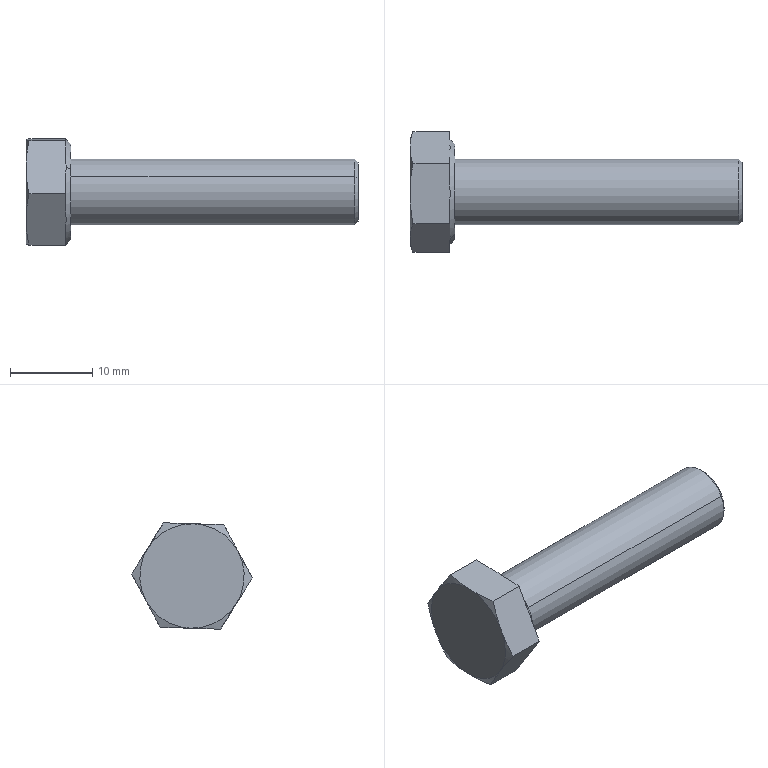Part | NX | features BREP 1 | 1 solid | 27 faces | box 40.45 x 14.692 x 12.962 mm | volume 2507 mm3 | plane 15 | cone 10 | cylinder 2 | commonest cylinder face diameters 8 x2
STEP:
#1=CARTESIAN_POINT('',(711.845,-32.743,42.746));
#2=VERTEX_POINT('',#1);
#3=CARTESIAN_POINT('',(711.845,-39.092,46.141));
#4=VERTEX_POINT('',#3);
#5=CARTESIAN_POINT('',(711.845,-35.917,44.443));
#6=DIRECTION('',(1.,0.,0.));
#7=DIRECTION('',(0.,0.8818,-0.4716));
#8=AXIS2_PLACEMENT_3D('',#5,#6,#7);
#9=CIRCLE('',#8,3.6);
#10=EDGE_CURVE('',#2,#4,#9,.T.);
#11=ORIENTED_EDGE('',*,*,#10,.F.);
#12=CARTESIAN_POINT('',(711.445,-32.39,42.557));
#13=VERTEX_POINT('',#12);
#14=CARTESIAN_POINT('',(711.845,-32.743,42.746));
#15=DIRECTION('',(-0.7071,0.6235,-0.3335));
#16=VECTOR('',#15,1000.);
#17=LINE('',#14,#16);
#18=EDGE_CURVE('',#13,#2,#17,.F.);
#19=ORIENTED_EDGE('',*,*,#18,.F.);
#20=CARTESIAN_POINT('',(711.445,-39.444,46.33));
#21=VERTEX_POINT('',#20);
#22=CARTESIAN_POINT('',(711.445,-35.917,44.443));
#23=DIRECTION('',(-1.,0.,0.));
#24=DIRECTION('',(0.,0.8818,-0.4716));
#25=AXIS2_PLACEMENT_3D('',#22,#23,#24);
#26=CIRCLE('',#25,4.);
#27=EDGE_CURVE('',#21,#13,#26,.T.);
#28=ORIENTED_EDGE('',*,*,#27,.F.);
#29=CARTESIAN_POINT('',(711.845,-39.092,46.141));
#30=DIRECTION('',(-0.7071,-0.6235,0.3335));
#31=VECTOR('',#30,1000.);
#32=LINE('',#29,#31);
#33=EDGE_CURVE('',#21,#4,#32,.F.);
#34=ORIENTED_EDGE('',*,*,#33,.T.);
#35=EDGE_LOOP('',(#11,#19,#28,#34));
#36=FACE_BOUND('',#35,.T.);
#37=CARTESIAN_POINT('',(711.845,-35.917,44.443));
#38=DIRECTION('',(-1.,0.,0.));
#39=DIRECTION('',(0.,0.8818,-0.4716));
#40=AXIS2_PLACEMENT_3D('',#37,#38,#39);
#41=CONICAL_SURFACE('',#40,3.6,0.7854);
#42=ADVANCED_FACE('',(#36),#41,.T.);
#43=ORIENTED_EDGE('',*,*,#27,.T.);
#44=CARTESIAN_POINT('',(676.845,-32.39,42.557));
#45=VERTEX_POINT('',#44);
#46=CARTESIAN_POINT('',(711.845,-32.39,42.557));
#47=DIRECTION('',(-1.,0.,0.));
#48=VECTOR('',#47,1000.);
#49=LINE('',#46,#48);
#50=EDGE_CURVE('',#45,#13,#49,.F.);
#51=ORIENTED_EDGE('',*,*,#50,.F.);
#52=CARTESIAN_POINT('',(676.845,-39.444,46.33));
#53=VERTEX_POINT('',#52);
#54=CARTESIAN_POINT('',(676.845,-35.917,44.443));
#55=DIRECTION('',(1.,0.,0.));
#56=DIRECTION('',(0.,0.8818,-0.4716));
#57=AXIS2_PLACEMENT_3D('',#54,#55,#56);
#58=CIRCLE('',#57,4.);
#59=EDGE_CURVE('',#45,#53,#58,.T.);
#60=ORIENTED_EDGE('',*,*,#59,.T.);
#61=CARTESIAN_POINT('',(711.845,-39.444,46.33));
#62=DIRECTION('',(-1.,0.,0.));
#63=VECTOR('',#62,1000.);
#64=LINE('',#61,#63);
#65=EDGE_CURVE('',#53,#21,#64,.F.);
#66=ORIENTED_EDGE('',*,*,#65,.T.);
#67=EDGE_LOOP('',(#43,#51,#60,#66));
#68=FACE_BOUND('',#67,.T.);
#69=CARTESIAN_POINT('',(711.845,-35.917,44.443));
#70=DIRECTION('',(-1.,0.,0.));
#71=DIRECTION('',(0.,0.8818,-0.4716));
#72=AXIS2_PLACEMENT_3D('',#69,#70,#71);
#73=CYLINDRICAL_SURFACE('',#72,4.);
#74=ADVANCED_FACE('',(#68),#73,.T.);
#75=CARTESIAN_POINT('',(676.845,-41.045,47.185));
#76=VERTEX_POINT('',#75);
#77=CARTESIAN_POINT('',(676.845,-30.789,41.701));
#78=VERTEX_POINT('',#77);
#79=CARTESIAN_POINT('',(676.845,-35.917,44.443));
#80=DIRECTION('',(-1.,0.,0.));
#81=DIRECTION('',(0.,-0.8818,0.4716));
#82=AXIS2_PLACEMENT_3D('',#79,#80,#81);
#83=CIRCLE('',#82,5.815);
#84=EDGE_CURVE('',#76,#78,#83,.T.);
#85=ORIENTED_EDGE('',*,*,#84,.T.);
#86=CARTESIAN_POINT('',(676.295,-30.304,41.442));
#87=VERTEX_POINT('',#86);
#88=CARTESIAN_POINT('',(676.245,-30.26,41.418));
#89=DIRECTION('',(-0.7071,0.6235,-0.3335));
#90=VECTOR('',#89,1000.);
#91=LINE('',#88,#90);
#92=EDGE_CURVE('',#87,#78,#91,.F.);
#93=ORIENTED_EDGE('',*,*,#92,.F.);
#94=CARTESIAN_POINT('',(676.245,-29.927,42.147));
#95=VERTEX_POINT('',#94);
#96=CARTESIAN_POINT('',(676.295,-30.304,41.442));
#97=CARTESIAN_POINT('',(676.295,-30.179,41.677));
#98=CARTESIAN_POINT('',(676.278,-30.053,41.912));
#99=CARTESIAN_POINT('',(676.245,-29.927,42.147));
#100=B_SPLINE_CURVE_WITH_KNOTS('',3,(#96,#97,#98,#99),.UNSPECIFIED.,.F.,.F.,(4,4),(0.,1.),.PIECEWISE_BEZIER_KNOTS.);
#101=EDGE_CURVE('',#87,#95,#100,.T.);
#102=ORIENTED_EDGE('',*,*,#101,.T.);
#103=CARTESIAN_POINT('',(676.245,-30.089,47.124));
#104=VERTEX_POINT('',#103);
#105=CARTESIAN_POINT('',(676.245,-35.917,44.443));
#106=DIRECTION('',(-1.,0.,0.));
#107=DIRECTION('',(0.,-0.8818,0.4716));
#108=AXIS2_PLACEMENT_3D('',#105,#106,#107);
#109=CIRCLE('',#108,6.415);
#110=EDGE_CURVE('',#104,#95,#109,.T.);
#111=ORIENTED_EDGE('',*,*,#110,.F.);
#112=CARTESIAN_POINT('',(676.245,-30.933,48.482));
#113=VERTEX_POINT('',#112);
#114=CARTESIAN_POINT('',(676.245,-30.089,47.124));
#115=CARTESIAN_POINT('',(676.311,-30.371,47.577));
#116=CARTESIAN_POINT('',(676.311,-30.652,48.03));
#117=CARTESIAN_POINT('',(676.245,-30.933,48.482));
#118=B_SPLINE_CURVE_WITH_KNOTS('',3,(#114,#115,#116,#117),.UNSPECIFIED.,.F.,.F.,(4,4),(0.,0.001599),.UNSPECIFIED.);
#119=EDGE_CURVE('',#104,#113,#118,.T.);
#120=ORIENTED_EDGE('',*,*,#119,.T.);
#121=CARTESIAN_POINT('',(676.245,-35.325,50.831));
#122=VERTEX_POINT('',#121);
#123=CARTESIAN_POINT('',(676.245,-35.917,44.443));
#124=DIRECTION('',(-1.,0.,0.));
#125=DIRECTION('',(0.,-0.8818,0.4716));
#126=AXIS2_PLACEMENT_3D('',#123,#124,#125);
#127=CIRCLE('',#126,6.415);
#128=EDGE_CURVE('',#122,#113,#127,.T.);
#129=ORIENTED_EDGE('',*,*,#128,.F.);
#130=CARTESIAN_POINT('',(676.245,-36.923,50.779));
#131=VERTEX_POINT('',#130);
#132=CARTESIAN_POINT('',(676.245,-35.325,50.831));
#133=CARTESIAN_POINT('',(676.311,-35.858,50.814));
#134=CARTESIAN_POINT('',(676.311,-36.391,50.796));
#135=CARTESIAN_POINT('',(676.245,-36.923,50.779));
#136=B_SPLINE_CURVE_WITH_KNOTS('',3,(#132,#133,#134,#135),.UNSPECIFIED.,.F.,.F.,(4,4),(0.,0.001599),.UNSPECIFIED.);
#137=EDGE_CURVE('',#122,#131,#136,.T.);
#138=ORIENTED_EDGE('',*,*,#137,.T.);
#139=CARTESIAN_POINT('',(676.245,-41.153,48.15));
#140=VERTEX_POINT('',#139);
#141=CARTESIAN_POINT('',(676.245,-35.917,44.443));
#142=DIRECTION('',(-1.,0.,0.));
#143=DIRECTION('',(0.,-0.8818,0.4716));
#144=AXIS2_PLACEMENT_3D('',#141,#142,#143);
#145=CIRCLE('',#144,6.415);
#146=EDGE_CURVE('',#140,#131,#145,.T.);
#147=ORIENTED_EDGE('',*,*,#146,.F.);
#148=CARTESIAN_POINT('',(676.295,-41.53,47.445));
#149=VERTEX_POINT('',#148);
#150=CARTESIAN_POINT('',(676.245,-41.153,48.15));
#151=CARTESIAN_POINT('',(676.278,-41.279,47.915));
#152=CARTESIAN_POINT('',(676.295,-41.404,47.68));
#153=CARTESIAN_POINT('',(676.295,-41.53,47.445));
#154=B_SPLINE_CURVE_WITH_KNOTS('',3,(#150,#151,#152,#153),.UNSPECIFIED.,.F.,.F.,(4,4),(0.,1.),.PIECEWISE_BEZIER_KNOTS.);
#155=EDGE_CURVE('',#140,#149,#154,.T.);
#156=ORIENTED_EDGE('',*,*,#155,.T.);
#157=CARTESIAN_POINT('',(676.245,-41.574,47.468));
#158=DIRECTION('',(-0.7071,-0.6235,0.3335));
#159=VECTOR('',#158,1000.);
#160=LINE('',#157,#159);
#161=EDGE_CURVE('',#149,#76,#160,.F.);
#162=ORIENTED_EDGE('',*,*,#161,.T.);
#163=EDGE_LOOP('',(#85,#93,#102,#111,#120,#129,#138,#147,#156,#162));
#164=FACE_BOUND('',#163,.T.);
#165=CARTESIAN_POINT('',(676.245,-35.917,44.443));
#166=DIRECTION('',(-1.,0.,0.));
#167=DIRECTION('',(0.,0.8818,-0.4716));
#168=AXIS2_PLACEMENT_3D('',#165,#166,#167);
#169=CONICAL_SURFACE('',#168,6.415,0.7854);
#170=ADVANCED_FACE('',(#164),#169,.T.);
#171=ORIENTED_EDGE('',*,*,#84,.F.);
#172=CARTESIAN_POINT('',(676.845,-35.917,44.443));
#173=DIRECTION('',(-1.,0.,0.));
#174=DIRECTION('',(0.,-0.8818,0.4716));
#175=AXIS2_PLACEMENT_3D('',#172,#173,#174);
#176=CIRCLE('',#175,5.815);
#177=EDGE_CURVE('',#78,#76,#176,.T.);
#178=ORIENTED_EDGE('',*,*,#177,.F.);
#179=EDGE_LOOP('',(#171,#178));
#180=FACE_BOUND('',#179,.T.);
#181=CARTESIAN_POINT('',(676.845,-35.917,44.443));
#182=DIRECTION('',(1.,0.,0.));
#183=DIRECTION('',(0.,0.8818,-0.4716));
#184=AXIS2_PLACEMENT_3D('',#181,#182,#183);
#185=CIRCLE('',#184,4.);
#186=EDGE_CURVE('',#53,#45,#185,.T.);
#187=ORIENTED_EDGE('',*,*,#186,.F.);
#188=ORIENTED_EDGE('',*,*,#59,.F.);
#189=EDGE_LOOP('',(#187,#188));
#190=FACE_BOUND('',#189,.T.);
#191=CARTESIAN_POINT('',(676.845,-32.037,38.201));
#192=DIRECTION('',(1.,0.,0.));
#193=DIRECTION('',(0.,-0.8818,0.4716));
#194=AXIS2_PLACEMENT_3D('',#191,#192,#193);
#195=PLANE('',#194);
#196=ADVANCED_FACE('',(#180,#190),#195,.T.);
#197=CARTESIAN_POINT('',(671.753,-32.037,38.201));
#198=VERTEX_POINT('',#197);
#199=CARTESIAN_POINT('',(671.395,-35.71,38.082));
#200=VERTEX_POINT('',#199);
#201=CARTESIAN_POINT('',(671.753,-32.037,38.201));
#202=CARTESIAN_POINT('',(671.532,-33.252,38.162));
#203=CARTESIAN_POINT('',(671.395,-34.474,38.122));
#204=CARTESIAN_POINT('',(671.395,-35.71,38.082));
#205=B_SPLINE_CURVE_WITH_KNOTS('',3,(#201,#202,#203,#204),.UNSPECIFIED.,.F.,.F.,(4,4),(0.,0.003692),.UNSPECIFIED.);
#206=EDGE_CURVE('',#198,#200,#205,.T.);
#207=ORIENTED_EDGE('',*,*,#206,.F.);
#208=CARTESIAN_POINT('',(676.245,-32.037,38.201));
#209=VERTEX_POINT('',#208);
#210=CARTESIAN_POINT('',(676.845,-32.037,38.201));
#211=DIRECTION('',(-1.,0.,0.));
#212=VECTOR('',#211,1000.);
#213=LINE('',#210,#212);
#214=EDGE_CURVE('',#209,#198,#213,.T.);
#215=ORIENTED_EDGE('',*,*,#214,.F.);
#216=CARTESIAN_POINT('',(676.245,-34.911,38.108));
#217=VERTEX_POINT('',#216);
#218=CARTESIAN_POINT('',(676.245,-39.383,37.962));
#219=DIRECTION('',(0.,0.9995,0.03252));
#220=VECTOR('',#219,1000.);
#221=LINE('',#218,#220);
#222=EDGE_CURVE('',#217,#209,#221,.T.);
#223=ORIENTED_EDGE('',*,*,#222,.F.);
#224=CARTESIAN_POINT('',(676.245,-36.509,38.056));
#225=VERTEX_POINT('',#224);
#226=CARTESIAN_POINT('',(676.245,-36.509,38.056));
#227=CARTESIAN_POINT('',(676.311,-35.976,38.073));
#228=CARTESIAN_POINT('',(676.311,-35.444,38.09));
#229=CARTESIAN_POINT('',(676.245,-34.911,38.108));
#230=B_SPLINE_CURVE_WITH_KNOTS('',3,(#226,#227,#228,#229),.UNSPECIFIED.,.F.,.F.,(4,4),(0.,0.001599),.UNSPECIFIED.);
#231=EDGE_CURVE('',#225,#217,#230,.T.);
#232=ORIENTED_EDGE('',*,*,#231,.F.);
#233=CARTESIAN_POINT('',(676.245,-39.383,37.962));
#234=VERTEX_POINT('',#233);
#235=CARTESIAN_POINT('',(676.245,-39.383,37.962));
#236=DIRECTION('',(0.,0.9995,0.03252));
#237=VECTOR('',#236,1000.);
#238=LINE('',#235,#237);
#239=EDGE_CURVE('',#234,#225,#238,.T.);
#240=ORIENTED_EDGE('',*,*,#239,.F.);
#241=CARTESIAN_POINT('',(671.753,-39.383,37.962));
#242=VERTEX_POINT('',#241);
#243=CARTESIAN_POINT('',(676.845,-39.383,37.962));
#244=DIRECTION('',(-1.,0.,0.));
#245=VECTOR('',#244,1000.);
#246=LINE('',#243,#245);
#247=EDGE_CURVE('',#234,#242,#246,.T.);
#248=ORIENTED_EDGE('',*,*,#247,.T.);
#249=CARTESIAN_POINT('',(671.395,-35.71,38.082));
#250=CARTESIAN_POINT('',(671.395,-36.946,38.041));
#251=CARTESIAN_POINT('',(671.532,-38.169,38.002));
#252=CARTESIAN_POINT('',(671.753,-39.383,37.962));
#253=B_SPLINE_CURVE_WITH_KNOTS('',3,(#249,#250,#251,#252),.UNSPECIFIED.,.F.,.F.,(4,4),(0.,0.003692),.UNSPECIFIED.);
#254=EDGE_CURVE('',#200,#242,#253,.T.);
#255=ORIENTED_EDGE('',*,*,#254,.F.);
#256=EDGE_LOOP('',(#207,#215,#223,#232,#240,#248,#255));
#257=FACE_BOUND('',#256,.T.);
#258=CARTESIAN_POINT('',(676.845,-39.383,37.962));
#259=DIRECTION('',(0.,-0.03252,0.9995));
#260=DIRECTION('',(0.,0.9995,0.03252));
#261=AXIS2_PLACEMENT_3D('',#258,#259,#260);
#262=PLANE('',#261);
#263=ADVANCED_FACE('',(#257),#262,.F.);
#264=CARTESIAN_POINT('',(671.753,-28.571,44.682));
#265=VERTEX_POINT('',#264);
#266=CARTESIAN_POINT('',(671.395,-30.304,41.442));
#267=VERTEX_POINT('',#266);
#268=CARTESIAN_POINT('',(671.753,-28.571,44.682));
#269=CARTESIAN_POINT('',(671.532,-29.144,43.611));
#270=CARTESIAN_POINT('',(671.395,-29.721,42.532));
#271=CARTESIAN_POINT('',(671.395,-30.304,41.442));
#272=B_SPLINE_CURVE_WITH_KNOTS('',3,(#268,#269,#270,#271),.UNSPECIFIED.,.F.,.F.,(4,4),(0.,0.003692),.UNSPECIFIED.);
#273=EDGE_CURVE('',#265,#267,#272,.T.);
#274=ORIENTED_EDGE('',*,*,#273,.F.);
#275=CARTESIAN_POINT('',(676.245,-28.571,44.682));
#276=VERTEX_POINT('',#275);
#277=CARTESIAN_POINT('',(676.845,-28.571,44.682));
#278=DIRECTION('',(-1.,0.,0.));
#279=VECTOR('',#278,1000.);
#280=LINE('',#277,#279);
#281=EDGE_CURVE('',#276,#265,#280,.T.);
#282=ORIENTED_EDGE('',*,*,#281,.F.);
#283=CARTESIAN_POINT('',(676.245,-32.037,38.201));
#284=DIRECTION('',(0.,0.4716,0.8818));
#285=VECTOR('',#284,1000.);
#286=LINE('',#283,#285);
#287=EDGE_CURVE('',#95,#276,#286,.T.);
#288=ORIENTED_EDGE('',*,*,#287,.F.);
#289=ORIENTED_EDGE('',*,*,#101,.F.);
#290=CARTESIAN_POINT('',(676.245,-30.681,40.737));
#291=VERTEX_POINT('',#290);
#292=CARTESIAN_POINT('',(676.245,-30.681,40.737));
#293=CARTESIAN_POINT('',(676.278,-30.556,40.972));
#294=CARTESIAN_POINT('',(676.295,-30.43,41.207));
#295=CARTESIAN_POINT('',(676.295,-30.304,41.442));
#296=B_SPLINE_CURVE_WITH_KNOTS('',3,(#292,#293,#294,#295),.UNSPECIFIED.,.F.,.F.,(4,4),(0.,1.),.PIECEWISE_BEZIER_KNOTS.);
#297=EDGE_CURVE('',#291,#87,#296,.T.);
#298=ORIENTED_EDGE('',*,*,#297,.F.);
#299=CARTESIAN_POINT('',(676.245,-32.037,38.201));
#300=DIRECTION('',(0.,0.4716,0.8818));
#301=VECTOR('',#300,1000.);
#302=LINE('',#299,#301);
#303=EDGE_CURVE('',#209,#291,#302,.T.);
#304=ORIENTED_EDGE('',*,*,#303,.F.);
#305=ORIENTED_EDGE('',*,*,#214,.T.);
#306=CARTESIAN_POINT('',(671.395,-30.304,41.442));
#307=CARTESIAN_POINT('',(671.395,-30.887,40.351));
#308=CARTESIAN_POINT('',(671.532,-31.464,39.273));
#309=CARTESIAN_POINT('',(671.753,-32.037,38.201));
#310=B_SPLINE_CURVE_WITH_KNOTS('',3,(#306,#307,#308,#309),.UNSPECIFIED.,.F.,.F.,(4,4),(0.,0.003692),.UNSPECIFIED.);
#311=EDGE_CURVE('',#267,#198,#310,.T.);
#312=ORIENTED_EDGE('',*,*,#311,.F.);
#313=EDGE_LOOP('',(#274,#282,#288,#289,#298,#304,#305,#312));
#314=FACE_BOUND('',#313,.T.);
#315=CARTESIAN_POINT('',(676.845,-32.037,38.201));
#316=DIRECTION('',(0.,-0.8818,0.4716));
#317=DIRECTION('',(-1.,0.,0.));
#318=AXIS2_PLACEMENT_3D('',#315,#316,#317);
#319=PLANE('',#318);
#320=ADVANCED_FACE('',(#314),#319,.F.);
#321=CARTESIAN_POINT('',(671.753,-32.451,50.924));
#322=VERTEX_POINT('',#321);
#323=CARTESIAN_POINT('',(671.395,-30.511,47.803));
#324=VERTEX_POINT('',#323);
#325=CARTESIAN_POINT('',(671.753,-32.451,50.924));
#326=CARTESIAN_POINT('',(671.532,-31.81,49.893));
#327=CARTESIAN_POINT('',(671.395,-31.164,48.854));
#328=CARTESIAN_POINT('',(671.395,-30.511,47.803));
#329=B_SPLINE_CURVE_WITH_KNOTS('',3,(#325,#326,#327,#328),.UNSPECIFIED.,.F.,.F.,(4,4),(0.,0.003692),.UNSPECIFIED.);
#330=EDGE_CURVE('',#322,#324,#329,.T.);
#331=ORIENTED_EDGE('',*,*,#330,.F.);
#332=CARTESIAN_POINT('',(676.245,-32.451,50.924));
#333=VERTEX_POINT('',#332);
#334=CARTESIAN_POINT('',(676.845,-32.451,50.924));
#335=DIRECTION('',(-1.,0.,0.));
#336=VECTOR('',#335,1000.);
#337=LINE('',#334,#336);
#338=EDGE_CURVE('',#333,#322,#337,.T.);
#339=ORIENTED_EDGE('',*,*,#338,.F.);
#340=CARTESIAN_POINT('',(676.245,-28.571,44.682));
#341=DIRECTION('',(0.,-0.5279,0.8493));
#342=VECTOR('',#341,1000.);
#343=LINE('',#340,#342);
#344=EDGE_CURVE('',#113,#333,#343,.T.);
#345=ORIENTED_EDGE('',*,*,#344,.F.);
#346=ORIENTED_EDGE('',*,*,#119,.F.);
#347=CARTESIAN_POINT('',(676.245,-28.571,44.682));
#348=DIRECTION('',(0.,-0.5279,0.8493));
#349=VECTOR('',#348,1000.);
#350=LINE('',#347,#349);
#351=EDGE_CURVE('',#276,#104,#350,.T.);
#352=ORIENTED_EDGE('',*,*,#351,.F.);
#353=ORIENTED_EDGE('',*,*,#281,.T.);
#354=CARTESIAN_POINT('',(671.395,-30.511,47.803));
#355=CARTESIAN_POINT('',(671.395,-29.859,46.753));
#356=CARTESIAN_POINT('',(671.532,-29.213,45.714));
#357=CARTESIAN_POINT('',(671.753,-28.571,44.682));
#358=B_SPLINE_CURVE_WITH_KNOTS('',3,(#354,#355,#356,#357),.UNSPECIFIED.,.F.,.F.,(4,4),(0.,0.003692),.UNSPECIFIED.);
#359=EDGE_CURVE('',#324,#265,#358,.T.);
#360=ORIENTED_EDGE('',*,*,#359,.F.);
#361=EDGE_LOOP('',(#331,#339,#345,#346,#352,#353,#360));
#362=FACE_BOUND('',#361,.T.);
#363=CARTESIAN_POINT('',(676.845,-28.571,44.682));
#364=DIRECTION('',(0.,-0.8493,-0.5279));
#365=DIRECTION('',(0.,-0.5279,0.8493));
#366=AXIS2_PLACEMENT_3D('',#363,#364,#365);
#367=PLANE('',#366);
#368=ADVANCED_FACE('',(#362),#367,.F.);
#369=CARTESIAN_POINT('',(671.753,-39.797,50.685));
#370=VERTEX_POINT('',#369);
#371=CARTESIAN_POINT('',(671.395,-36.124,50.805));
#372=VERTEX_POINT('',#371);
#373=CARTESIAN_POINT('',(671.753,-39.797,50.685));
#374=CARTESIAN_POINT('',(671.532,-38.583,50.725));
#375=CARTESIAN_POINT('',(671.395,-37.36,50.765));
#376=CARTESIAN_POINT('',(671.395,-36.124,50.805));
#377=B_SPLINE_CURVE_WITH_KNOTS('',3,(#373,#374,#375,#376),.UNSPECIFIED.,.F.,.F.,(4,4),(0.,0.003692),.UNSPECIFIED.);
#378=EDGE_CURVE('',#370,#372,#377,.T.);
#379=ORIENTED_EDGE('',*,*,#378,.F.);
#380=CARTESIAN_POINT('',(676.245,-39.797,50.685));
#381=VERTEX_POINT('',#380);
#382=CARTESIAN_POINT('',(676.845,-39.797,50.685));
#383=DIRECTION('',(-1.,0.,0.));
#384=VECTOR('',#383,1000.);
#385=LINE('',#382,#384);
#386=EDGE_CURVE('',#381,#370,#385,.T.);
#387=ORIENTED_EDGE('',*,*,#386,.F.);
#388=CARTESIAN_POINT('',(676.245,-32.451,50.924));
#389=DIRECTION('',(0.,-0.9995,-0.03252));
#390=VECTOR('',#389,1000.);
#391=LINE('',#388,#390);
#392=EDGE_CURVE('',#131,#381,#391,.T.);
#393=ORIENTED_EDGE('',*,*,#392,.F.);
#394=ORIENTED_EDGE('',*,*,#137,.F.);
#395=CARTESIAN_POINT('',(676.245,-32.451,50.924));
#396=DIRECTION('',(0.,-0.9995,-0.03252));
#397=VECTOR('',#396,1000.);
#398=LINE('',#395,#397);
#399=EDGE_CURVE('',#333,#122,#398,.T.);
#400=ORIENTED_EDGE('',*,*,#399,.F.);
#401=ORIENTED_EDGE('',*,*,#338,.T.);
#402=CARTESIAN_POINT('',(671.395,-36.124,50.805));
#403=CARTESIAN_POINT('',(671.395,-34.888,50.845));
#404=CARTESIAN_POINT('',(671.532,-33.666,50.885));
#405=CARTESIAN_POINT('',(671.753,-32.451,50.924));
#406=B_SPLINE_CURVE_WITH_KNOTS('',3,(#402,#403,#404,#405),.UNSPECIFIED.,.F.,.F.,(4,4),(0.,0.003692),.UNSPECIFIED.);
#407=EDGE_CURVE('',#372,#322,#406,.T.);
#408=ORIENTED_EDGE('',*,*,#407,.F.);
#409=EDGE_LOOP('',(#379,#387,#393,#394,#400,#401,#408));
#410=FACE_BOUND('',#409,.T.);
#411=CARTESIAN_POINT('',(676.845,-32.451,50.924));
#412=DIRECTION('',(0.,0.03252,-0.9995));
#413=DIRECTION('',(0.,-0.9995,-0.03252));
#414=AXIS2_PLACEMENT_3D('',#411,#412,#413);
#415=PLANE('',#414);
#416=ADVANCED_FACE('',(#410),#415,.F.);
#417=CARTESIAN_POINT('',(671.753,-43.263,44.204));
#418=VERTEX_POINT('',#417);
#419=CARTESIAN_POINT('',(671.395,-41.53,47.445));
#420=VERTEX_POINT('',#419);
#421=CARTESIAN_POINT('',(671.753,-43.263,44.204));
#422=CARTESIAN_POINT('',(671.532,-42.69,45.276));
#423=CARTESIAN_POINT('',(671.395,-42.113,46.354));
#424=CARTESIAN_POINT('',(671.395,-41.53,47.445));
#425=B_SPLINE_CURVE_WITH_KNOTS('',3,(#421,#422,#423,#424),.UNSPECIFIED.,.F.,.F.,(4,4),(0.,0.003692),.UNSPECIFIED.);
#426=EDGE_CURVE('',#418,#420,#425,.T.);
#427=ORIENTED_EDGE('',*,*,#426,.F.);
#428=CARTESIAN_POINT('',(676.245,-43.263,44.204));
#429=VERTEX_POINT('',#428);
#430=CARTESIAN_POINT('',(676.845,-43.263,44.204));
#431=DIRECTION('',(-1.,0.,0.));
#432=VECTOR('',#431,1000.);
#433=LINE('',#430,#432);
#434=EDGE_CURVE('',#429,#418,#433,.T.);
#435=ORIENTED_EDGE('',*,*,#434,.F.);
#436=CARTESIAN_POINT('',(676.245,-41.907,46.74));
#437=VERTEX_POINT('',#436);
#438=CARTESIAN_POINT('',(676.245,-39.797,50.685));
#439=DIRECTION('',(0.,-0.4716,-0.8818));
#440=VECTOR('',#439,1000.);
#441=LINE('',#438,#440);
#442=EDGE_CURVE('',#437,#429,#441,.T.);
#443=ORIENTED_EDGE('',*,*,#442,.F.);
#444=CARTESIAN_POINT('',(676.295,-41.53,47.445));
#445=CARTESIAN_POINT('',(676.295,-41.656,47.21));
#446=CARTESIAN_POINT('',(676.278,-41.781,46.975));
#447=CARTESIAN_POINT('',(676.245,-41.907,46.74));
#448=B_SPLINE_CURVE_WITH_KNOTS('',3,(#444,#445,#446,#447),.UNSPECIFIED.,.F.,.F.,(4,4),(0.,1.),.PIECEWISE_BEZIER_KNOTS.);
#449=EDGE_CURVE('',#149,#437,#448,.T.);
#450=ORIENTED_EDGE('',*,*,#449,.F.);
#451=ORIENTED_EDGE('',*,*,#155,.F.);
#452=CARTESIAN_POINT('',(676.245,-39.797,50.685));
#453=DIRECTION('',(0.,-0.4716,-0.8818));
#454=VECTOR('',#453,1000.);
#455=LINE('',#452,#454);
#456=EDGE_CURVE('',#381,#140,#455,.T.);
#457=ORIENTED_EDGE('',*,*,#456,.F.);
#458=ORIENTED_EDGE('',*,*,#386,.T.);
#459=CARTESIAN_POINT('',(671.395,-41.53,47.445));
#460=CARTESIAN_POINT('',(671.395,-40.947,48.535));
#461=CARTESIAN_POINT('',(671.532,-40.37,49.614));
#462=CARTESIAN_POINT('',(671.753,-39.797,50.685));
#463=B_SPLINE_CURVE_WITH_KNOTS('',3,(#459,#460,#461,#462),.UNSPECIFIED.,.F.,.F.,(4,4),(0.,0.003692),.UNSPECIFIED.);
#464=EDGE_CURVE('',#420,#370,#463,.T.);
#465=ORIENTED_EDGE('',*,*,#464,.F.);
#466=EDGE_LOOP('',(#427,#435,#443,#450,#451,#457,#458,#465));
#467=FACE_BOUND('',#466,.T.);
#468=CARTESIAN_POINT('',(676.845,-39.797,50.685));
#469=DIRECTION('',(0.,0.8818,-0.4716));
#470=DIRECTION('',(1.,0.,0.));
#471=AXIS2_PLACEMENT_3D('',#468,#469,#470);
#472=PLANE('',#471);
#473=ADVANCED_FACE('',(#467),#472,.F.);
#474=CARTESIAN_POINT('',(671.395,-41.323,41.083));
#475=VERTEX_POINT('',#474);
#476=CARTESIAN_POINT('',(671.753,-39.383,37.962));
#477=CARTESIAN_POINT('',(671.532,-40.024,38.994));
#478=CARTESIAN_POINT('',(671.395,-40.67,40.033));
#479=CARTESIAN_POINT('',(671.395,-41.323,41.083));
#480=B_SPLINE_CURVE_WITH_KNOTS('',3,(#476,#477,#478,#479),.UNSPECIFIED.,.F.,.F.,(4,4),(0.,0.003692),.UNSPECIFIED.);
#481=EDGE_CURVE('',#242,#475,#480,.T.);
#482=ORIENTED_EDGE('',*,*,#481,.F.);
#483=ORIENTED_EDGE('',*,*,#247,.F.);
#484=CARTESIAN_POINT('',(676.245,-40.901,40.404));
#485=VERTEX_POINT('',#484);
#486=CARTESIAN_POINT('',(676.245,-43.263,44.204));
#487=DIRECTION('',(0.,0.5279,-0.8493));
#488=VECTOR('',#487,1000.);
#489=LINE('',#486,#488);
#490=EDGE_CURVE('',#485,#234,#489,.T.);
#491=ORIENTED_EDGE('',*,*,#490,.F.);
#492=CARTESIAN_POINT('',(676.245,-41.745,41.762));
#493=VERTEX_POINT('',#492);
#494=CARTESIAN_POINT('',(676.245,-41.745,41.762));
#495=CARTESIAN_POINT('',(676.311,-41.464,41.31));
#496=CARTESIAN_POINT('',(676.311,-41.182,40.857));
#497=CARTESIAN_POINT('',(676.245,-40.901,40.404));
#498=B_SPLINE_CURVE_WITH_KNOTS('',3,(#494,#495,#496,#497),.UNSPECIFIED.,.F.,.F.,(4,4),(0.,0.001599),.UNSPECIFIED.);
#499=EDGE_CURVE('',#493,#485,#498,.T.);
#500=ORIENTED_EDGE('',*,*,#499,.F.);
#501=CARTESIAN_POINT('',(676.245,-43.263,44.204));
#502=DIRECTION('',(0.,0.5279,-0.8493));
#503=VECTOR('',#502,1000.);
#504=LINE('',#501,#503);
#505=EDGE_CURVE('',#429,#493,#504,.T.);
#506=ORIENTED_EDGE('',*,*,#505,.F.);
#507=ORIENTED_EDGE('',*,*,#434,.T.);
#508=CARTESIAN_POINT('',(671.395,-41.323,41.083));
#509=CARTESIAN_POINT('',(671.395,-41.976,42.133));
#510=CARTESIAN_POINT('',(671.532,-42.622,43.172));
#511=CARTESIAN_POINT('',(671.753,-43.263,44.204));
#512=B_SPLINE_CURVE_WITH_KNOTS('',3,(#508,#509,#510,#511),.UNSPECIFIED.,.F.,.F.,(4,4),(0.,0.003692),.UNSPECIFIED.);
#513=EDGE_CURVE('',#475,#418,#512,.T.);
#514=ORIENTED_EDGE('',*,*,#513,.F.);
#515=EDGE_LOOP('',(#482,#483,#491,#500,#506,#507,#514));
#516=FACE_BOUND('',#515,.T.);
#517=CARTESIAN_POINT('',(676.845,-43.263,44.204));
#518=DIRECTION('',(0.,0.8493,0.5279));
#519=DIRECTION('',(0.,0.5279,-0.8493));
#520=AXIS2_PLACEMENT_3D('',#517,#518,#519);
#521=PLANE('',#520);
#522=ADVANCED_FACE('',(#516),#521,.F.);
#523=ORIENTED_EDGE('',*,*,#222,.T.);
#524=ORIENTED_EDGE('',*,*,#303,.T.);
#525=CARTESIAN_POINT('',(676.245,-35.917,44.443));
#526=DIRECTION('',(-1.,0.,0.));
#527=DIRECTION('',(0.,-0.8818,0.4716));
#528=AXIS2_PLACEMENT_3D('',#525,#526,#527);
#529=CIRCLE('',#528,6.415);
#530=EDGE_CURVE('',#291,#217,#529,.T.);
#531=ORIENTED_EDGE('',*,*,#530,.T.);
#532=EDGE_LOOP('',(#523,#524,#531));
#533=FACE_BOUND('',#532,.T.);
#534=CARTESIAN_POINT('',(676.245,-32.892,50.1));
#535=DIRECTION('',(1.,0.,0.));
#536=DIRECTION('',(0.,-0.8818,0.4716));
#537=AXIS2_PLACEMENT_3D('',#534,#535,#536);
#538=PLANE('',#537);
#539=ADVANCED_FACE('',(#533),#538,.T.);
#540=ORIENTED_EDGE('',*,*,#287,.T.);
#541=ORIENTED_EDGE('',*,*,#351,.T.);
#542=ORIENTED_EDGE('',*,*,#110,.T.);
#543=EDGE_LOOP('',(#540,#541,#542));
#544=FACE_BOUND('',#543,.T.);
#545=CARTESIAN_POINT('',(676.245,-32.892,50.1));
#546=DIRECTION('',(1.,0.,0.));
#547=DIRECTION('',(0.,-0.8818,0.4716));
#548=AXIS2_PLACEMENT_3D('',#545,#546,#547);
#549=PLANE('',#548);
#550=ADVANCED_FACE('',(#544),#549,.T.);
#551=ORIENTED_EDGE('',*,*,#344,.T.);
#552=ORIENTED_EDGE('',*,*,#399,.T.);
#553=ORIENTED_EDGE('',*,*,#128,.T.);
#554=EDGE_LOOP('',(#551,#552,#553));
#555=FACE_BOUND('',#554,.T.);
#556=CARTESIAN_POINT('',(676.245,-32.892,50.1));
#557=DIRECTION('',(1.,0.,0.));
#558=DIRECTION('',(0.,-0.8818,0.4716));
#559=AXIS2_PLACEMENT_3D('',#556,#557,#558);
#560=PLANE('',#559);
#561=ADVANCED_FACE('',(#555),#560,.T.);
#562=ORIENTED_EDGE('',*,*,#392,.T.);
#563=ORIENTED_EDGE('',*,*,#456,.T.);
#564=ORIENTED_EDGE('',*,*,#146,.T.);
#565=EDGE_LOOP('',(#562,#563,#564));
#566=FACE_BOUND('',#565,.T.);
#567=CARTESIAN_POINT('',(676.245,-32.892,50.1));
#568=DIRECTION('',(1.,0.,0.));
#569=DIRECTION('',(0.,-0.8818,0.4716));
#570=AXIS2_PLACEMENT_3D('',#567,#568,#569);
#571=PLANE('',#570);
#572=ADVANCED_FACE('',(#566),#571,.T.);
#573=ORIENTED_EDGE('',*,*,#442,.T.);
#574=ORIENTED_EDGE('',*,*,#505,.T.);
#575=CARTESIAN_POINT('',(676.245,-35.917,44.443));
#576=DIRECTION('',(-1.,0.,0.));
#577=DIRECTION('',(0.,-0.8818,0.4716));
#578=AXIS2_PLACEMENT_3D('',#575,#576,#577);
#579=CIRCLE('',#578,6.415);
#580=EDGE_CURVE('',#493,#437,#579,.T.);
#581=ORIENTED_EDGE('',*,*,#580,.T.);
#582=EDGE_LOOP('',(#573,#574,#581));
#583=FACE_BOUND('',#582,.T.);
#584=CARTESIAN_POINT('',(676.245,-32.892,50.1));
#585=DIRECTION('',(1.,0.,0.));
#586=DIRECTION('',(0.,-0.8818,0.4716));
#587=AXIS2_PLACEMENT_3D('',#584,#585,#586);
#588=PLANE('',#587);
#589=ADVANCED_FACE('',(#583),#588,.T.);
#590=ORIENTED_EDGE('',*,*,#239,.T.);
#591=CARTESIAN_POINT('',(676.245,-35.917,44.443));
#592=DIRECTION('',(-1.,0.,0.));
#593=DIRECTION('',(0.,-0.8818,0.4716));
#594=AXIS2_PLACEMENT_3D('',#591,#592,#593);
#595=CIRCLE('',#594,6.415);
#596=EDGE_CURVE('',#225,#485,#595,.T.);
#597=ORIENTED_EDGE('',*,*,#596,.T.);
#598=ORIENTED_EDGE('',*,*,#490,.T.);
#599=EDGE_LOOP('',(#590,#597,#598));
#600=FACE_BOUND('',#599,.T.);
#601=CARTESIAN_POINT('',(676.245,-32.892,50.1));
#602=DIRECTION('',(1.,0.,0.));
#603=DIRECTION('',(0.,-0.8818,0.4716));
#604=AXIS2_PLACEMENT_3D('',#601,#602,#603);
#605=PLANE('',#604);
#606=ADVANCED_FACE('',(#600),#605,.T.);
#607=ORIENTED_EDGE('',*,*,#92,.T.);
#608=ORIENTED_EDGE('',*,*,#177,.T.);
#609=ORIENTED_EDGE('',*,*,#161,.F.);
#610=ORIENTED_EDGE('',*,*,#449,.T.);
#611=ORIENTED_EDGE('',*,*,#580,.F.);
#612=ORIENTED_EDGE('',*,*,#499,.T.);
#613=ORIENTED_EDGE('',*,*,#596,.F.);
#614=ORIENTED_EDGE('',*,*,#231,.T.);
#615=ORIENTED_EDGE('',*,*,#530,.F.);
#616=ORIENTED_EDGE('',*,*,#297,.T.);
#617=EDGE_LOOP('',(#607,#608,#609,#610,#611,#612,#613,#614,#615,#616));
#618=FACE_BOUND('',#617,.T.);
#619=CARTESIAN_POINT('',(676.245,-35.917,44.443));
#620=DIRECTION('',(-1.,0.,0.));
#621=DIRECTION('',(0.,0.8818,-0.4716));
#622=AXIS2_PLACEMENT_3D('',#619,#620,#621);
#623=CONICAL_SURFACE('',#622,6.415,0.7854);
#624=ADVANCED_FACE('',(#618),#623,.T.);
#625=ORIENTED_EDGE('',*,*,#311,.T.);
#626=ORIENTED_EDGE('',*,*,#206,.T.);
#627=CARTESIAN_POINT('',(671.395,-35.917,44.443));
#628=DIRECTION('',(1.,0.,0.));
#629=DIRECTION('',(0.,0.8818,-0.4716));
#630=AXIS2_PLACEMENT_3D('',#627,#628,#629);
#631=CIRCLE('',#630,6.365);
#632=EDGE_CURVE('',#200,#267,#631,.T.);
#633=ORIENTED_EDGE('',*,*,#632,.T.);
#634=EDGE_LOOP('',(#625,#626,#633));
#635=FACE_BOUND('',#634,.T.);
#636=CARTESIAN_POINT('',(671.395,-35.917,44.443));
#637=DIRECTION('',(1.,0.,0.));
#638=DIRECTION('',(0.,-0.8818,0.4716));
#639=AXIS2_PLACEMENT_3D('',#636,#637,#638);
#640=CONICAL_SURFACE('',#639,6.365,1.222);
#641=ADVANCED_FACE('',(#635),#640,.T.);
#642=ORIENTED_EDGE('',*,*,#254,.T.);
#643=ORIENTED_EDGE('',*,*,#481,.T.);
#644=CARTESIAN_POINT('',(671.395,-35.917,44.443));
#645=DIRECTION('',(1.,0.,0.));
#646=DIRECTION('',(0.,0.8818,-0.4716));
#647=AXIS2_PLACEMENT_3D('',#644,#645,#646);
#648=CIRCLE('',#647,6.365);
#649=EDGE_CURVE('',#475,#200,#648,.T.);
#650=ORIENTED_EDGE('',*,*,#649,.T.);
#651=EDGE_LOOP('',(#642,#643,#650));
#652=FACE_BOUND('',#651,.T.);
#653=CARTESIAN_POINT('',(671.395,-35.917,44.443));
#654=DIRECTION('',(1.,0.,0.));
#655=DIRECTION('',(0.,-0.8818,0.4716));
#656=AXIS2_PLACEMENT_3D('',#653,#654,#655);
#657=CONICAL_SURFACE('',#656,6.365,1.222);
#658=ADVANCED_FACE('',(#652),#657,.T.);
#659=ORIENTED_EDGE('',*,*,#426,.T.);
#660=CARTESIAN_POINT('',(671.395,-35.917,44.443));
#661=DIRECTION('',(1.,0.,0.));
#662=DIRECTION('',(0.,0.8818,-0.4716));
#663=AXIS2_PLACEMENT_3D('',#660,#661,#662);
#664=CIRCLE('',#663,6.365);
#665=EDGE_CURVE('',#420,#475,#664,.T.);
#666=ORIENTED_EDGE('',*,*,#665,.T.);
#667=ORIENTED_EDGE('',*,*,#513,.T.);
#668=EDGE_LOOP('',(#659,#666,#667));
#669=FACE_BOUND('',#668,.T.);
#670=CARTESIAN_POINT('',(671.395,-35.917,44.443));
#671=DIRECTION('',(1.,0.,0.));
#672=DIRECTION('',(0.,-0.8818,0.4716));
#673=AXIS2_PLACEMENT_3D('',#670,#671,#672);
#674=CONICAL_SURFACE('',#673,6.365,1.222);
#675=ADVANCED_FACE('',(#669),#674,.T.);
#676=ORIENTED_EDGE('',*,*,#378,.T.);
#677=CARTESIAN_POINT('',(671.395,-35.917,44.443));
#678=DIRECTION('',(-1.,0.,0.));
#679=DIRECTION('',(0.,-0.8818,0.4716));
#680=AXIS2_PLACEMENT_3D('',#677,#678,#679);
#681=CIRCLE('',#680,6.365);
#682=EDGE_CURVE('',#420,#372,#681,.T.);
#683=ORIENTED_EDGE('',*,*,#682,.F.);
#684=ORIENTED_EDGE('',*,*,#464,.T.);
#685=EDGE_LOOP('',(#676,#683,#684));
#686=FACE_BOUND('',#685,.T.);
#687=CARTESIAN_POINT('',(671.395,-35.917,44.443));
#688=DIRECTION('',(1.,0.,0.));
#689=DIRECTION('',(0.,-0.8818,0.4716));
#690=AXIS2_PLACEMENT_3D('',#687,#688,#689);
#691=CONICAL_SURFACE('',#690,6.365,1.222);
#692=ADVANCED_FACE('',(#686),#691,.T.);
#693=ORIENTED_EDGE('',*,*,#330,.T.);
#694=CARTESIAN_POINT('',(671.395,-35.917,44.443));
#695=DIRECTION('',(1.,0.,0.));
#696=DIRECTION('',(0.,0.8818,-0.4716));
#697=AXIS2_PLACEMENT_3D('',#694,#695,#696);
#698=CIRCLE('',#697,6.365);
#699=EDGE_CURVE('',#324,#372,#698,.T.);
#700=ORIENTED_EDGE('',*,*,#699,.T.);
#701=ORIENTED_EDGE('',*,*,#407,.T.);
#702=EDGE_LOOP('',(#693,#700,#701));
#703=FACE_BOUND('',#702,.T.);
#704=CARTESIAN_POINT('',(671.395,-35.917,44.443));
#705=DIRECTION('',(1.,0.,0.));
#706=DIRECTION('',(0.,-0.8818,0.4716));
#707=AXIS2_PLACEMENT_3D('',#704,#705,#706);
#708=CONICAL_SURFACE('',#707,6.365,1.222);
#709=ADVANCED_FACE('',(#703),#708,.T.);
#710=ORIENTED_EDGE('',*,*,#359,.T.);
#711=ORIENTED_EDGE('',*,*,#273,.T.);
#712=CARTESIAN_POINT('',(671.395,-35.917,44.443));
#713=DIRECTION('',(1.,0.,0.));
#714=DIRECTION('',(0.,0.8818,-0.4716));
#715=AXIS2_PLACEMENT_3D('',#712,#713,#714);
#716=CIRCLE('',#715,6.365);
#717=EDGE_CURVE('',#267,#324,#716,.T.);
#718=ORIENTED_EDGE('',*,*,#717,.T.);
#719=EDGE_LOOP('',(#710,#711,#718));
#720=FACE_BOUND('',#719,.T.);
#721=CARTESIAN_POINT('',(671.395,-35.917,44.443));
#722=DIRECTION('',(1.,0.,0.));
#723=DIRECTION('',(0.,-0.8818,0.4716));
#724=AXIS2_PLACEMENT_3D('',#721,#722,#723);
#725=CONICAL_SURFACE('',#724,6.365,1.222);
#726=ADVANCED_FACE('',(#720),#725,.T.);
#727=ORIENTED_EDGE('',*,*,#717,.F.);
#728=ORIENTED_EDGE('',*,*,#632,.F.);
#729=ORIENTED_EDGE('',*,*,#649,.F.);
#730=ORIENTED_EDGE('',*,*,#665,.F.);
#731=ORIENTED_EDGE('',*,*,#682,.T.);
#732=ORIENTED_EDGE('',*,*,#699,.F.);
#733=EDGE_LOOP('',(#727,#728,#729,#730,#731,#732));
#734=FACE_BOUND('',#733,.T.);
#735=CARTESIAN_POINT('',(671.395,-32.037,38.201));
#736=DIRECTION('',(1.,0.,0.));
#737=DIRECTION('',(0.,-0.8818,0.4716));
#738=AXIS2_PLACEMENT_3D('',#735,#736,#737);
#739=PLANE('',#738);
#740=ADVANCED_FACE('',(#734),#739,.F.);
#741=ORIENTED_EDGE('',*,*,#50,.T.);
#742=CARTESIAN_POINT('',(711.445,-35.917,44.443));
#743=DIRECTION('',(-1.,0.,0.));
#744=DIRECTION('',(0.,0.8818,-0.4716));
#745=AXIS2_PLACEMENT_3D('',#742,#743,#744);
#746=CIRCLE('',#745,4.);
#747=EDGE_CURVE('',#13,#21,#746,.T.);
#748=ORIENTED_EDGE('',*,*,#747,.T.);
#749=ORIENTED_EDGE('',*,*,#65,.F.);
#750=ORIENTED_EDGE('',*,*,#186,.T.);
#751=EDGE_LOOP('',(#741,#748,#749,#750));
#752=FACE_BOUND('',#751,.T.);
#753=CARTESIAN_POINT('',(711.845,-35.917,44.443));
#754=DIRECTION('',(-1.,0.,0.));
#755=DIRECTION('',(0.,0.8818,-0.4716));
#756=AXIS2_PLACEMENT_3D('',#753,#754,#755);
#757=CYLINDRICAL_SURFACE('',#756,4.);
#758=ADVANCED_FACE('',(#752),#757,.T.);
#759=CARTESIAN_POINT('',(711.845,-35.917,44.443));
#760=DIRECTION('',(1.,0.,0.));
#761=DIRECTION('',(0.,0.8818,-0.4716));
#762=AXIS2_PLACEMENT_3D('',#759,#760,#761);
#763=CIRCLE('',#762,3.6);
#764=EDGE_CURVE('',#4,#2,#763,.T.);
#765=ORIENTED_EDGE('',*,*,#764,.T.);
#766=ORIENTED_EDGE('',*,*,#10,.T.);
#767=EDGE_LOOP('',(#765,#766));
#768=FACE_BOUND('',#767,.T.);
#769=CARTESIAN_POINT('',(711.845,-35.917,44.443));
#770=DIRECTION('',(1.,0.,0.));
#771=DIRECTION('',(0.,-0.8818,0.4716));
#772=AXIS2_PLACEMENT_3D('',#769,#770,#771);
#773=PLANE('',#772);
#774=ADVANCED_FACE('',(#768),#773,.T.);
#775=ORIENTED_EDGE('',*,*,#18,.T.);
#776=ORIENTED_EDGE('',*,*,#764,.F.);
#777=ORIENTED_EDGE('',*,*,#33,.F.);
#778=ORIENTED_EDGE('',*,*,#747,.F.);
#779=EDGE_LOOP('',(#775,#776,#777,#778));
#780=FACE_BOUND('',#779,.T.);
#781=CARTESIAN_POINT('',(711.845,-35.917,44.443));
#782=DIRECTION('',(-1.,0.,0.));
#783=DIRECTION('',(0.,0.8818,-0.4716));
#784=AXIS2_PLACEMENT_3D('',#781,#782,#783);
#785=CONICAL_SURFACE('',#784,3.6,0.7854);
#786=ADVANCED_FACE('',(#780),#785,.T.);
#787=CLOSED_SHELL('',(#42,#74,#170,#196,#263,#320,#368,#416,#473,#522,#539,#550,#561,#572,#589,#606,#624,#641,#658,#675,#692,#709,#726,#740,#758,#774,#786));
#788=MANIFOLD_SOLID_BREP('',#787);
#789=(LENGTH_UNIT()NAMED_UNIT(*)SI_UNIT(.MILLI.,.METRE.));
#790=UNCERTAINTY_MEASURE_WITH_UNIT(LENGTH_MEASURE(0.0508),#789,'','');
#791=(NAMED_UNIT(*)PLANE_ANGLE_UNIT()SI_UNIT($,.RADIAN.));
#792=(NAMED_UNIT(*)SI_UNIT($,.STERADIAN.)SOLID_ANGLE_UNIT());
#793=(GEOMETRIC_REPRESENTATION_CONTEXT(3)GLOBAL_UNCERTAINTY_ASSIGNED_CONTEXT((#790))GLOBAL_UNIT_ASSIGNED_CONTEXT((#789,#791,#792))REPRESENTATION_CONTEXT('',''));
#794=ADVANCED_BREP_SHAPE_REPRESENTATION('',(#788),#793);